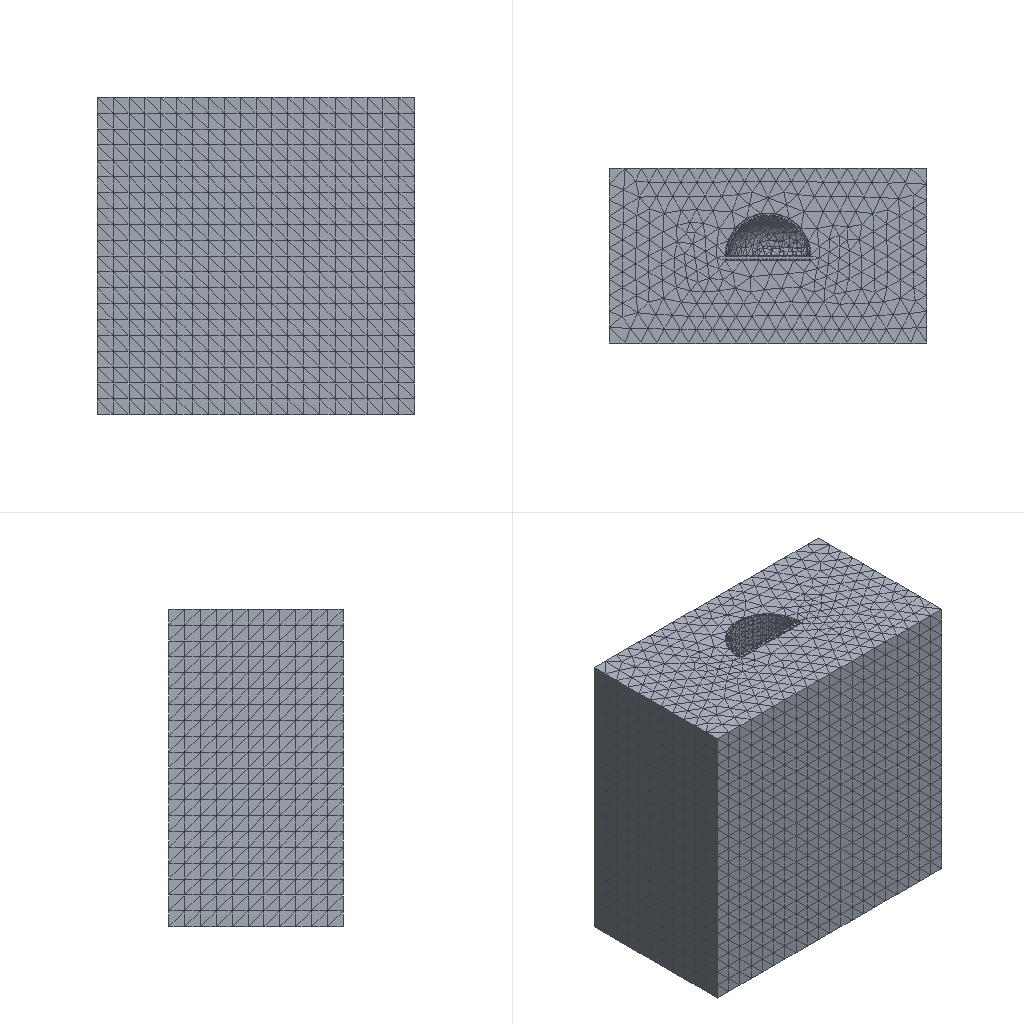Simulation study | abaqus
Set-up summary:
category,name,step,type,value,unit,region
solver,abaqus
solver,version,,,Abaqus/Standard 2020
units,not stated in the deck,,not stated
analysis,deck,,static,static
load_step,Step-1,Step-1,static
load_step,requested,,,1
mesh,nodes,,,64756
mesh,elements,,,42991
element_type,S4R,,shell,5090
element_type,C3D10,,solid,37901
load,load commands in deck,,count,2
bc,support commands in deck,,count,3
material,CONCRETE,,in results
material,REBAR,,in results
material,SOIL,,in results
check,setup vs results,,match,"per instance, exact: element labels, types and connectivity; labels of the nodes the elements use; coordinates of those nodes at SINGLE_PRECISION in 1 of 4 instance(s)"
Abaqus input file, long lists of numbers shortened:
*Heading
** Job name: Job-4 Model name: Model-1-Copy
** Generated by: Abaqus/CAE 2020
*Preprint, echo=NO, model=NO, history=NO, contact=NO
**
** PARTS
**
*Part, name=Part-1
*Node
      1,   2.7,   1.2,  0.3
      2,   2.7,          1.5,  0.3
** (45226 more lines like these left out)
*Element, type=C3D10
    1,  2088,  2089,  2090,  2091,  6178,  6177,  6176,  6180,  6179,  6181
    2,  2088,  2092,  2093,  2094,  6184,  6183,  6182,  6186,  6185,  6187
** (30789 more lines like these left out)
*Nset, nset=Set-11, generate
     1,  45228,      1
*Elset, elset=Set-11, generate
     1,  30791,      1
** Section: Section-1-soil
*Solid Section, elset=Set-11, material=soil
,
*End Part
**
*Part, name=con
*Node
      1,   6.717,   1.55,           0.
      2,   1.717,   1.55,           0.
** (14123 more lines like these left out)
*Element, type=C3D10
   1,   216,  1104,   217,   384,  2362,  2361,  2360,  2364,  2363,  2365
   2,   217,  2298,  2072,  1104,  2368,  2367,  2366,  2361,  2369,  2370
** (7108 more lines like these left out)
*Nset, nset=Set-5, generate
     1,  14125,      1
*Elset, elset=Set-5, generate
    1,  7110,     1
** Section: Section-2-concrete
*Solid Section, elset=Set-5, material=concrete
,
*End Part
**
*Part, name=jin-zhixian
*Node
      1,   14.37,   1.487, -0.215
      2,   14.37,    6.702, -0.215
** (1602 more lines like these left out)
*Element, type=S4R
  1,   1,  21, 335,  82
  2,  21,  22, 336, 335
** (1472 more lines like these left out)
*Nset, nset=Set-1
    3,    4,    5,    6,    7,    8,    9,   10,   13,   14,   15,   16,   17,   18,   19,   20
   52,   53,   54,   55,   56,   57,   58,   59,   60,   61,   62,   63,   64,   83,   84,   85
** (63 more lines like these left out)
*Elset, elset=Set-1
  267,  268,  269,  270,  271,  272,  273,  274,  275,  276,  277,  278,  279,  280,  281,  282
  283,  284,  285,  286,  287,  288,  289,  290,  291,  292,  293,  294,  295,  296,  297,  298
** (57 more lines like these left out)
*Nset, nset=Set-3, generate
    1,  1604,     1
*Elset, elset=Set-3, generate
    1,  1474,     1
** Section: rebar
*Shell Section, elset=Set-3, material=rebar
0.001, 5
*End Part
**
*Part, name=xian-wanqu
*Node
      1,   12.382,   8.64,           0.
      2,   12.382,   3.53,           0.
** (3797 more lines like these left out)
*Element, type=S4R
  1,    1,   21,  522,  118
  2,   21,   22,  523,  522
** (3614 more lines like these left out)
*Nset, nset=Set-1
    3,    4,    5,    6,    7,    8,    9,   10,   13,   14,   15,   16,   17,   18,   19,   20
   70,   71,   72,   73,   74,   75,   76,   77,   78,   79,   80,   81,   82,   83,   84,   85
** (150 more lines like these left out)
*Elset, elset=Set-1
  649,  650,  651,  652,  653,  654,  655,  656,  657,  658,  659,  660,  661,  662,  663,  664
  665,  666,  667,  668,  669,  670,  671,  672,  673,  674,  675,  676,  677,  678,  679,  680
** (142 more lines like these left out)
*Nset, nset=Set-3, generate
    1,  3799,     1
*Elset, elset=Set-3, generate
    1,  3616,     1
** Section: rebar
*Shell Section, elset=Set-3, material=rebar
0.001, 5
*End Part
**
**
** ASSEMBLY
**
*Assembly, name=Assembly
**
*Instance, name=Part-1-1, part=Part-1
*End Instance
**
*Instance, name=con-1, part=con
    -4.217,          1.5,     7.25
    -4.217,          1.5,     7.25, -5.217,          1.5,     7.25, 90.
*End Instance
**
*Instance, name=xian-wanqu-1, part=xian-wanqu
   -2.382,          1.5,      9.085
   -2.382,          1.5,      9.085, -3.382,          1.5,      9.085, 90.
*End Instance
**
*Instance, name=jin-zhixian-1, part=jin-zhixian
   -4.373,        1.505,     7.097
   -4.373,        1.505,     7.097, -5.373,        1.505,     7.097, 90.
*End Instance
**
*Nset, nset=Set-13, instance=Part-1-1
     6,     7,     8,     9,    19,    20,    21,    22,    23,    24,    25,    26,    27,    28,    29,    30
    31,    32,    33,    34,    79,    80,    81,    82,    83,    84,    85,    86,   103,   104,   105,   106
** (128 more lines like these left out)
*Nset, nset=Set-13, instance=con-1
    23,    24,    25,    26,    27,    28,   279,   280,   281,   282,   283,   284,   285,   286,   287,   288
   317,   318,   319,   320,   321,   322,   323,   324,   325,   354,   355,   356,   357,   358,   359,   360
** (9 more lines like these left out)
*Elset, elset=Set-13, instance=Part-1-1
   128,   183,   225,   229,   332,   379,   440,   453,   559,   592,   722,   915,  1091,  1247,  1330,  1396
  1447,  1471,  1472,  1539,  1679,  1810,  1834,  1956,  1992,  2019,  2168,  2172,  2173,  2275,  2317,  2421
** (59 more lines like these left out)
*Elset, elset=Set-13, instance=con-1
  213,  812,  814,  815,  819,  821,  826,  832,  844,  846,  851,  861,  862,  864,  870,  880
  886,  887,  890,  902, 1518, 1527, 1533, 1876, 1949, 1965, 1974, 1998, 2031, 2036, 2047, 2052
** (2 more lines like these left out)
*Nset, nset=Set-14, instance=Part-1-1
    22,    23,    24,    25,    27,    32,    33,    34,   164,   165,   166,   167,   168,   169,   170,   171
   172,   173,   174,   175,   176,   177,   178,   179,   180,   226,   227,   228,   229,   230,   231,   232
** (104 more lines like these left out)
*Elset, elset=Set-14, instance=Part-1-1
   318,  1252,  2089,  2090,  2176,  2420,  2520,  2590,  2726,  2805,  2851,  2852,  2860,  2873,  2875,  2888
  2897,  2907,  2909,  2912,  2915,  2966,  2987,  2996,  2999,  3005,  3006,  3012,  3025,  3045,  3047,  3055
** (48 more lines like these left out)
*Nset, nset=Set-17, instance=Part-1-1, generate
     1,  45228,      1
*Elset, elset=Set-17, instance=Part-1-1, generate
     1,  30791,      1
*Nset, nset=Set-18, instance=Part-1-1
    12,    14,    16,    18,    21,    22,    25,    26,    27,    28,    29,    32,   119,   120,   121,   122
   135,   136,   137,   138,   139,   140,   141,   142,   154,   155,   156,   157,   158,   159,   160,   161
** (126 more lines like these left out)
*Nset, nset=Set-18, instance=con-1
     4,     6,     7,     8,     9,    10,    51,    52,    53,    54,    55,    56,    57,    58,    59,    88
    89,    90,    91,    92,    93,    94,    95,    96,    97,    98,    99,   100,   101,   102,   103,   104
** (9 more lines like these left out)
*Elset, elset=Set-18, instance=Part-1-1
   502,   548,   609,   722,   917,  1257,  1305,  1835,  2463,  2570,  2591,  2594,  2621,  2632,  2700,  2701
  2730,  2736,  2737,  2787,  2788,  2796,  2797,  2805,  2816,  2831,  2837,  2842,  2849,  2853,  2877,  2896
** (58 more lines like these left out)
*Elset, elset=Set-18, instance=con-1
 1417, 1579, 2498, 3696, 3741, 3975, 5114, 5152, 5161, 5169, 5175, 5199, 5205, 5217, 5227, 5237
 5244, 6259, 6271, 6414, 6462, 6552, 6556, 6565, 6591, 6592, 6598, 6612, 6633, 6636, 6639, 6650
** (2 more lines like these left out)
*Nset, nset=m_Set-10, instance=xian-wanqu-1
    3,    4,    5,    6,    7,    8,    9,   10,   13,   14,   15,   16,   17,   18,   19,   20
   70,   71,   72,   73,   74,   75,   76,   77,   78,   79,   80,   81,   82,   83,   84,   85
** (150 more lines like these left out)
*Elset, elset=m_Set-10, instance=xian-wanqu-1
  649,  650,  651,  652,  653,  654,  655,  656,  657,  658,  659,  660,  661,  662,  663,  664
  665,  666,  667,  668,  669,  670,  671,  672,  673,  674,  675,  676,  677,  678,  679,  680
** (142 more lines like these left out)
*Nset, nset=m_Set-15, instance=jin-zhixian-1
    3,    4,    5,    6,    7,    8,    9,   10,   13,   14,   15,   16,   17,   18,   19,   20
   52,   53,   54,   55,   56,   57,   58,   59,   60,   61,   62,   63,   64,   83,   84,   85
** (63 more lines like these left out)
*Elset, elset=m_Set-15, instance=jin-zhixian-1
  267,  268,  269,  270,  271,  272,  273,  274,  275,  276,  277,  278,  279,  280,  281,  282
  283,  284,  285,  286,  287,  288,  289,  290,  291,  292,  293,  294,  295,  296,  297,  298
** (57 more lines like these left out)
*Nset, nset=m_Set-19, instance=xian-wanqu-1, generate
    1,  3799,     1
*Nset, nset=m_Set-19, instance=jin-zhixian-1, generate
    1,  1604,     1
*Elset, elset=m_Set-19, instance=xian-wanqu-1, generate
    1,  3616,     1
*Elset, elset=m_Set-19, instance=jin-zhixian-1, generate
    1,  1474,     1
*Nset, nset=s_Set-10, instance=con-1, generate
     1,  14125,      1
*Elset, elset=s_Set-10, instance=con-1, generate
    1,  7110,     1
*Nset, nset=s_Set-15, instance=con-1, generate
     1,  14125,      1
*Elset, elset=s_Set-15, instance=con-1, generate
    1,  7110,     1
*Nset, nset=s_Set-19, instance=con-1, generate
     1,  14125,      1
*Elset, elset=s_Set-19, instance=con-1, generate
    1,  7110,     1
*Elset, elset=_Surf-4_S3, internal, instance=Part-1-1
    42,   502,  1465,  1514,  1566,  1643,  1717,  1950,  2503,  2553,  2580,  2583,  2586,  2625,  2663,  2692
  2699,  2703,  2727,  2735,  2740,  2753,  2768,  2784,  2791,  2815,  2827,  2856,  2933,  3015,  3035,  3051
** (45 more lines like these left out)
*Elset, elset=_Surf-4_S2, internal, instance=Part-1-1
  3574,  5379,  5451,  5895,  6212,  6382,  6723,  8370,  8478,  8891,  8894,  8896,  8989,  9333,  9417,  9862
 10045, 10165
*Elset, elset=_Surf-4_S1, internal, instance=Part-1-1
  5035,  5100,  5116,  5431,  5434,  6119,  6167,  6211,  6516,  7793,  8253,  9757,  9787, 17581, 20873, 22903
 26137,
*Elset, elset=_Surf-4_S4, internal, instance=Part-1-1
  5133,  5403,  8351,  8668,  8759,  9130,  9175,  9277,  9491, 10253, 10602, 10612, 11131, 13432, 13729, 15869
 17329, 20600, 20937, 24976, 26443, 26446
*Surface, type=ELEMENT, name=Surf-4
_Surf-4_S3, S3
_Surf-4_S2, S2
_Surf-4_S4, S4
_Surf-4_S1, S1
*Elset, elset=_m_Surf-2_S3, internal, instance=con-1
   23,   37,   70,   76,   79,  158,  161,  168,  172,  183,  189,  209,  249,  265,  373,  380
  388,  411,  420,  422,  426,  448,  468,  473,  483,  484,  487,  493,  513,  548,  550,  555
** (26 more lines like these left out)
*Elset, elset=_m_Surf-2_S1, internal, instance=con-1
   14,   16,   49,   59,   60,   62,   77,   80,   88,  109,  117,  134,  150,  152,  154,  171
  177,  187,  222,  264,  273,  275,  281,  283,  285,  291,  296,  305,  325,  327,  338,  354
** (40 more lines like these left out)
*Elset, elset=_m_Surf-2_S2, internal, instance=con-1
   10,   18,   38,   54,   78,   89,   90,  106,  121,  132,  133,  136,  137,  140,  141,  143
  148,  153,  166,  167,  181,  184,  188,  197,  202,  203,  205,  211,  217,  235,  245,  259
** (43 more lines like these left out)
*Elset, elset=_m_Surf-2_S4, internal, instance=con-1
    3,    7,   21,   24,   31,   35,   43,   67,   84,   92,   95,   96,  101,  110,  116,  135
  169,  174,  175,  212,  215,  218,  240,  246,  247,  256,  262,  270,  272,  280,  282,  290
** (37 more lines like these left out)
*Surface, type=ELEMENT, name=m_Surf-2
_m_Surf-2_S3, S3
_m_Surf-2_S1, S1
_m_Surf-2_S2, S2
_m_Surf-2_S4, S4
*Elset, elset=_s_Surf-2_S3, internal, instance=Part-1-1
    50,   259,   388,   717,   906,   920,   938,  1208,  1377,  1443,  1598,  1800,  2171,  2223,  2315,  2525
  2576,  2577,  2608,  2618,  2631,  2646,  2664,  2669,  2670,  2673,  2751,  2757,  2766,  2776,  2782,  2792
** (36 more lines like these left out)
*Elset, elset=_s_Surf-2_S2, internal, instance=Part-1-1
   190,  2869,  3214,  3317,  3356,  3529,  3636,  3711,  4020,  4281,  4536,  4557,  4558,  4614,  4808,  4970
  4999,  5055,  5083,  6847, 11326, 11965, 12315
*Elset, elset=_s_Surf-2_S4, internal, instance=Part-1-1
  3530,  3654,  3744,  3867,  4070,  4318,  5135,  8073, 10340, 11613, 11747, 12311, 14901, 15622, 15770, 19162
 19311, 20411, 21996, 22193, 23601, 23740, 24486
*Elset, elset=_s_Surf-2_S1, internal, instance=Part-1-1
  3552,  3572,  3907,  4163,  4572,  4678,  5129,  5879,  8734, 10018, 10537, 15389, 17368, 20143, 23264, 23462
 25029, 27401, 28532
*Surface, type=ELEMENT, name=s_Surf-2
_s_Surf-2_S3, S3
_s_Surf-2_S2, S2
_s_Surf-2_S4, S4
_s_Surf-2_S1, S1
** Constraint: Constraint-2
*Tie, name=Constraint-2, adjust=yes
s_Surf-2, m_Surf-2
** Constraint: Constraint-3
*Embedded Element, host elset=s_Set-19
m_Set-19
*End Assembly
*Amplitude, name=Amp-1
             0.,              0.,              1.,              1.
**
** MATERIALS
**
*Material, name=concrete
*Density
2500.,
*Elastic
 2.9791e+10, 0.2
*Concrete Damaged Plasticity
30.,    0.1,   1.16, 0.6667,   0.05
*Concrete Compression Hardening
 1.54e+07,      0.
 1.69e+07,  0.0002
 1.96e+07, 0.00048
 2.01e+07, 0.00079
    2e+07, 0.00095
 1.96e+07,  0.0011
 1.91e+07, 0.00127
 1.86e+07, 0.00143
 1.79e+07,  0.0016
 1.72e+07, 0.00177
 1.66e+07, 0.00194
 1.59e+07, 0.00211
 1.53e+07, 0.00228
 1.47e+07, 0.00245
 1.41e+07, 0.00261
 1.35e+07, 0.00278
  1.3e+07, 0.00294
 1.25e+07,  0.0031
  1.2e+07, 0.00327
 1.16e+07, 0.00343
 1.12e+07, 0.00359
 1.08e+07, 0.00375
 1.04e+07, 0.00391
 1.01e+07, 0.00406
*Concrete Tension Stiffening
 2.06e+06,      0.
 1.92e+06,   2e-05
 1.72e+06,   4e-05
 1.53e+06,   6e-05
 1.37e+06,   8e-05
 1.24e+06,  0.0001
 1.13e+06, 0.00011
 1.04e+06, 0.00013
  970000., 0.00015
  900000., 0.00016
  850000., 0.00018
*Concrete Compression Damage
     0.,      0.
 0.0841,   9e-05
 0.0933,  0.0001
 0.1091, 0.00013
 0.1418,  0.0002
 0.2407, 0.00048
  0.322, 0.00079
 0.3557, 0.00095
 0.3886,  0.0011
 0.4201, 0.00127
 0.4499, 0.00143
 0.4778,  0.0016
 0.5039, 0.00177
 0.5282, 0.00194
 0.5506, 0.00211
 0.5715, 0.00228
 0.5908, 0.00245
 0.6086, 0.00261
 0.6252, 0.00278
 0.6406, 0.00294
 0.6549,  0.0031
 0.6682, 0.00327
 0.6806, 0.00343
 0.6922, 0.00359
  0.703, 0.00375
 0.7131, 0.00391
 0.7227, 0.00406
   0.74, 0.00438
 0.7554, 0.00469
 0.7691,   0.005
 0.7815, 0.00531
 0.7926, 0.00561
 0.8026, 0.00592
 0.8118, 0.00622
 0.8202, 0.00653
 0.8278, 0.00683
 0.8349, 0.00713
*Concrete Tension Damage
      0.,      0.
 0.1181,   2e-05
 0.2281,   4e-05
 0.3187,   6e-05
 0.3919,   8e-05
 0.4512,  0.0001
 0.5, 0.00011
  0.5407, 0.00013
 0.575, 0.00015
 0.6043, 0.00016
 0.6297, 0.00018
 0.7177, 0.00025
 0.7702, 0.00033
 0.8053,  0.0004
 0.8304, 0.00047
 0.8494, 0.00054
  0.8643, 0.00061
 0.8763, 0.00068
 0.8862, 0.00075
*Material, name=rebar
*Density
7860.,
*Elastic
 2.1e+11, 0.3
*Material, name=soil
*Density
1800.,
*Elastic
 4.79e+07, 0.35
*Mohr Coulomb
25.,0.
*Mohr Coulomb Hardening
25000.,0.
**
** PREDEFINED FIELDS
**
** Name: Predefined Field-1   Type: Geostatic stress
*Initial Conditions, type=STRESS, GEOSTATIC
Set-17, 0., 6., -20000., -4., 2., 2.
** ----------------------------------------------------------------
**
** STEP: Step-1
**
*Step, name=Step-1, nlgeom=YES, inc=1000
*Static, stabilize=0.0002, allsdtol=0.05, continue=NO
0.01, 1., 1e-05, 1.
**
** BOUNDARY CONDITIONS
**
** Name: BC-1 Type: 位移/转角
*Boundary
Set-18, 3, 3
** Name: BC-2 Type: 位移/转角
*Boundary
Set-13, 1, 1
** Name: BC-3 Type: 位移/转角
*Boundary
Set-14, 2, 2
**
** LOADS
**
** Name: Load-2   Type: Pressure
*Dsload, amplitude=Amp-1
Surf-4, P, 1e+06
** Name: Load-3   Type: Gravity
*Dload
, GRAV, 9.8, 0., -1., 0.
**
** OUTPUT REQUESTS
**
*Restart, write, frequency=0
**
** FIELD OUTPUT: F-Output-1
**
*Output, field
*Node Output
CF, RF, RM, RT, TF, U, V
*Element Output, directions=YES
DAMAGEC, DAMAGET, E, LE, MISES, MISESMAX, PE, PEEQ, PEMAG, S, SDEG, SF, SSAVG
*Contact Output
CDISP, CSTRESS
**
** HISTORY OUTPUT: H-Output-1
**
*Output, history, variable=PRESELECT
*End Step
Results summary:
result,step,,completed,increments=51 time=1.0/1.0
result,analysis,,,static
result,last_loadstep,,,1
result,primary field,,,"U, UR"
result,reaction total,,FX,422285.857,model units
result,reaction total,,FY,474463935.551,model units
result,reaction total,,FZ,599571.836,model units